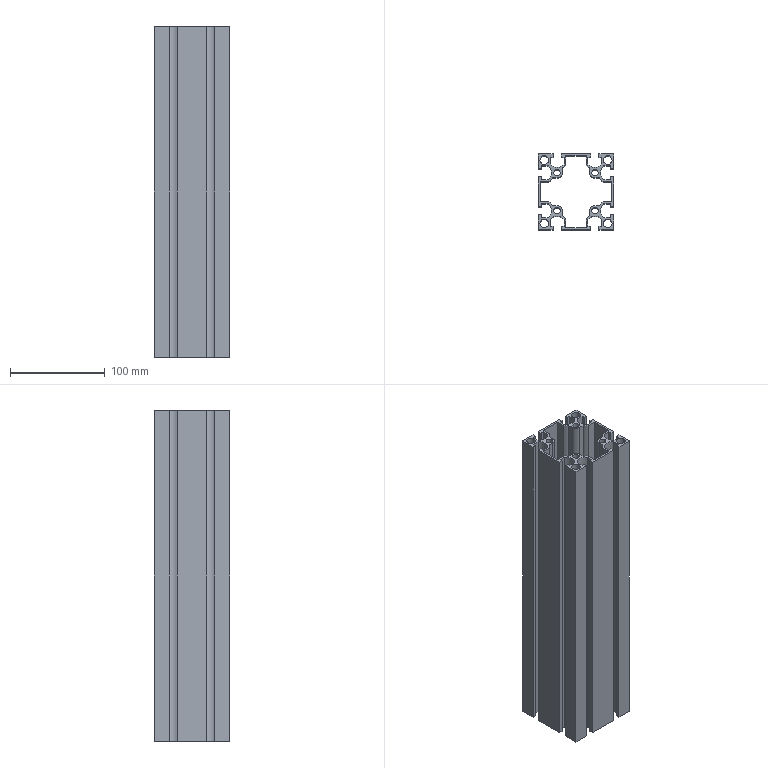Part | STEP file | 1 solid | 110 faces | box 80 x 80 x 350 mm | volume 477520 mm3 | plane 82 | cylinder 28 | commonest cylinder face diameters 19 x8 23 x8 6.8 x4 9.2 x4 10.8 x4